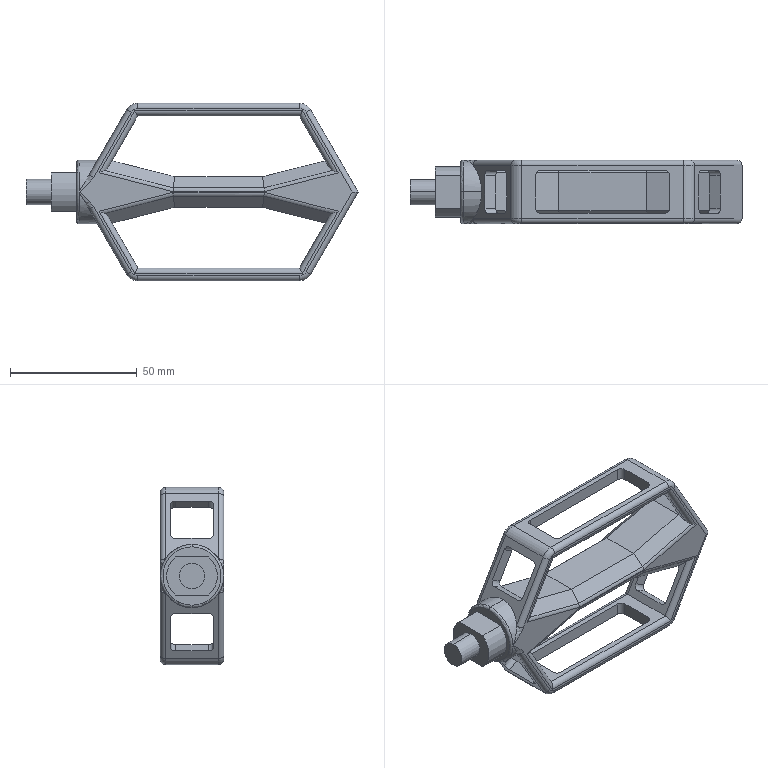Part | STEP file | Pedal Basic | 1 solid | 146 faces | box 131 x 25 x 70 mm | volume 58244 mm3 | cylinder 71 | plane 61 | torus 10 | spline 4 | commonest cylinder face diameters 4 x60 10 x6 25 x3 20 x2